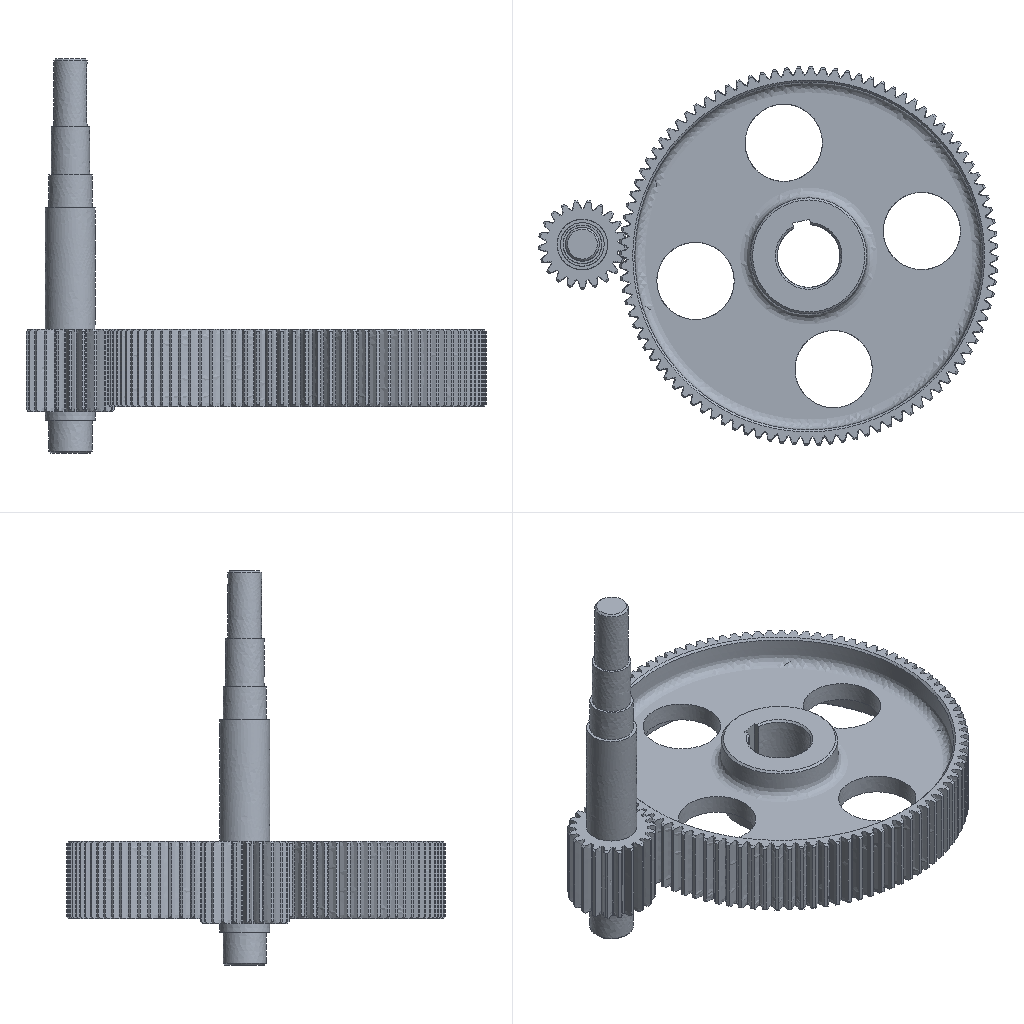Simulation study | ansys workbench
Set-up summary:
category,name,step,type,value,unit,region
solver,ansys_workbench
units,mm-N-s-tonne (MPa),,stated,"/units,MPA"
analysis,deck-1/LS1,,modal,method=lanb; n_modes=10
load_step,deck-1/LS1,deck-1/LS1,modal
analysis,deck-2/LS1,,modal,method=lanb; n_modes=10
load_step,deck-2/LS1,deck-2/LS1,modal
mesh,deck-1.dat,,nodes,219728
mesh,deck-1.dat,,elements,122793
element_type,SOLID187,,,122793,,deck-1.dat
mesh,deck-2.dat,,nodes,253520
mesh,deck-2.dat,,elements,144076
element_type,SOLID187,,,144076,,deck-2.dat
material,Structural Steel,,E,200000,tonne s^-2 mm^-1
material,Structural Steel,,nu,0.3
material,Structural Steel,,density,7.85e-09,tonne mm^-3
material,Structural Steel,,conductivity,60.5,tonne mm s^-3 C^-1
material,Structural Steel,,specific_heat,4.34e+08,mm^2 s^-2 C^-1
material,Structural Steel,,cte,1.2e-05,C^-1
material,Structural Steel,,permeability,10000
material,Structural Steel,,resistivity,0.00017,ohm mm
material,Structural Steel,,E,200000,tonne s^-2 mm^-1
material,Structural Steel,,nu,0.3
material,Structural Steel,,density,7.85e-09,tonne mm^-3
material,Structural Steel,,conductivity,60.5,tonne mm s^-3 C^-1
material,Structural Steel,,specific_heat,4.34e+08,mm^2 s^-2 C^-1
material,Structural Steel,,cte,1.2e-05,C^-1
material,Structural Steel,,permeability,10000
material,Structural Steel,,resistivity,0.00017,ohm mm
bc,Frictionless Supports X,deck-1/model,fixed,[dofs=UX],,_FRICSUX
bc,Frictionless Supports Z,deck-1/model,fixed,[dofs=UZ],,_FRICSUZ
bc,Frictionless Supports X,deck-2/model,fixed,[dofs=UX],,_FRICSUX
bc,Frictionless Supports Z,deck-2/model,fixed,[dofs=UZ],,_FRICSUZ
named_set,_FRICSUX,,node,8519
named_set,_FRICSUZ,,node,8519
named_set,_FRICSUX,,node,11532
named_set,_FRICSUZ,,node,11532
Results summary:
result,analyses[0].index,,,1
result,analyses[0].system,,,SYS
result,analyses[0].deck,,,deck-1.dat
result,analyses[0].solve_status,,,completed
result,analyses[0].analysis_type,,,modal
result,analyses[0].physics,,,mechanical
result,analyses[0].unit_system,,,"NMM: mm, ton, N, s, mV, mA, degC"
result,analyses[0].n_sets,,,10
result,analyses[0].modal_frequencies_hz[1],,,0
result,analyses[0].modal_frequencies_hz[2],,,0.001041
result,analyses[0].modal_frequencies_hz[3],,,532.799
result,analyses[0].modal_frequencies_hz[4],,,533.893
result,analyses[0].modal_frequencies_hz[5],,,691.53
result,analyses[0].modal_frequencies_hz[6],,,782.886
result,analyses[0].modal_frequencies_hz[7],,,802.65
result,analyses[0].modal_frequencies_hz[8],,,1382.87
result,analyses[0].modal_frequencies_hz[9],,,1387.25
result,analyses[0].modal_frequencies_hz[10],,,1917.86
result,analyses[1].index,,,2
result,analyses[1].system,,,SYS-1
result,analyses[1].deck,,,deck-2.dat
result,analyses[1].solve_status,,,completed
result,analyses[1].analysis_type,,,modal
result,analyses[1].physics,,,mechanical
result,analyses[1].unit_system,,,"NMM: mm, ton, N, s, mV, mA, degC"
result,analyses[1].n_sets,,,10
result,analyses[1].modal_frequencies_hz[1],,,0
result,analyses[1].modal_frequencies_hz[2],,,0
result,analyses[1].modal_frequencies_hz[3],,,478.151
result,analyses[1].modal_frequencies_hz[4],,,479.441
result,analyses[1].modal_frequencies_hz[5],,,662.317
result,analyses[1].modal_frequencies_hz[6],,,735.459
result,analyses[1].modal_frequencies_hz[7],,,741.336
result,analyses[1].modal_frequencies_hz[8],,,1855.63
result,analyses[1].modal_frequencies_hz[9],,,1855.86
result,analyses[1].modal_frequencies_hz[10],,,2443.72
result,geometry_export[0][0],,,1.step
result,geometry_export[0][1],,,ok
result,geometry_export[0][2],,,2
result,geometry_export[1][0],,,2.step
result,geometry_export[1][1],,,ok
result,geometry_export[1][2],,,2